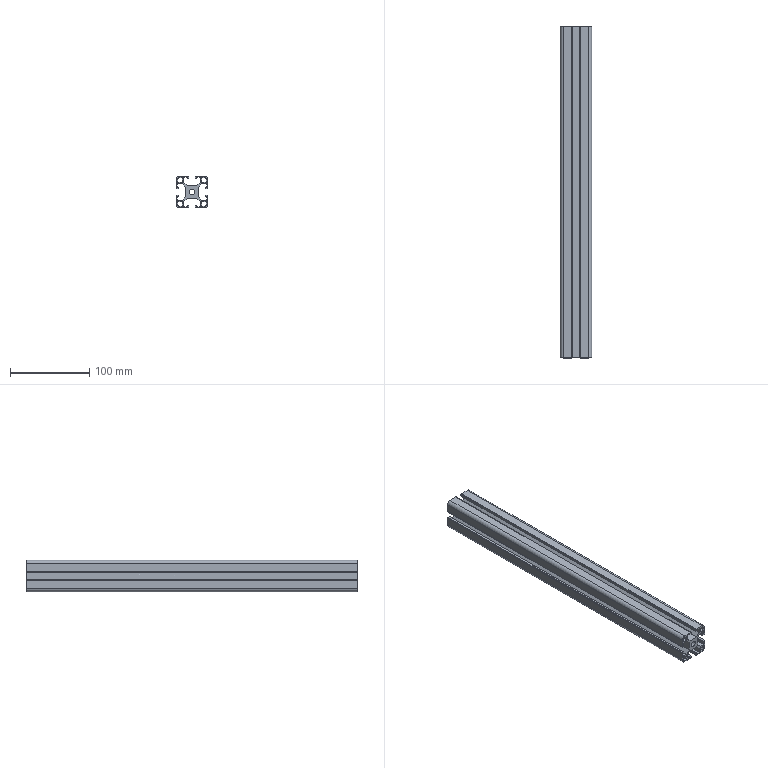Part | SolidWorks | features BaseBody 1 | 1 solid | 104 faces | box 40 x 420 x 40 mm | volume 242149 mm3 | plane 94 | cylinder 10 | commonest cylinder face diameters 5 x4 9 x4 6.8 x2